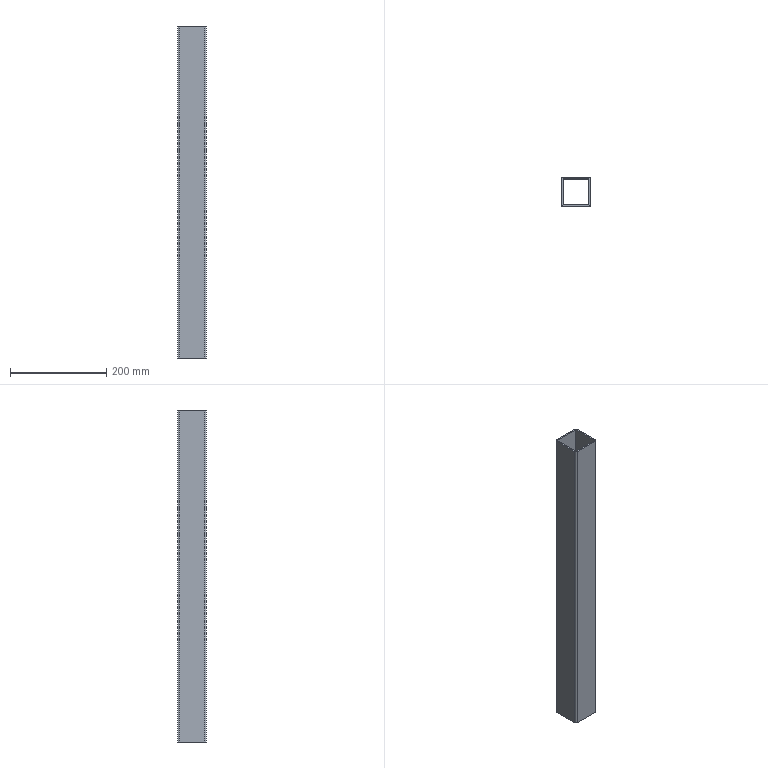Part | STEP file | X77-03104 | 1 solid | 14 faces | box 60 x 60 x 690 mm | volume 466629 mm3 | plane 10 | cylinder 4 | commonest cylinder face diameters 6 x4
STEP:
#1=CARTESIAN_POINT('',(0.,3.,690.));
#2=VERTEX_POINT('',#1);
#3=CARTESIAN_POINT('',(3.,0.,690.));
#4=VERTEX_POINT('',#3);
#5=CARTESIAN_POINT('',(3.,3.,690.));
#6=DIRECTION('',(0.,0.,1.));
#7=DIRECTION('',(1.,0.,0.));
#8=AXIS2_PLACEMENT_3D('',#5,#6,#7);
#9=CIRCLE('',#8,3.);
#10=EDGE_CURVE('',#2,#4,#9,.T.);
#11=ORIENTED_EDGE('',*,*,#10,.T.);
#12=CARTESIAN_POINT('',(57.,0.,690.));
#13=VERTEX_POINT('',#12);
#14=CARTESIAN_POINT('',(3.,0.,690.));
#15=DIRECTION('',(1.,0.,0.));
#16=VECTOR('',#15,1000.);
#17=LINE('',#14,#16);
#18=EDGE_CURVE('',#4,#13,#17,.T.);
#19=ORIENTED_EDGE('',*,*,#18,.T.);
#20=CARTESIAN_POINT('',(60.,3.,690.));
#21=VERTEX_POINT('',#20);
#22=CARTESIAN_POINT('',(57.,3.,690.));
#23=DIRECTION('',(0.,0.,1.));
#24=DIRECTION('',(1.,0.,0.));
#25=AXIS2_PLACEMENT_3D('',#22,#23,#24);
#26=CIRCLE('',#25,3.);
#27=EDGE_CURVE('',#13,#21,#26,.T.);
#28=ORIENTED_EDGE('',*,*,#27,.T.);
#29=CARTESIAN_POINT('',(60.,57.,690.));
#30=VERTEX_POINT('',#29);
#31=CARTESIAN_POINT('',(60.,3.,690.));
#32=DIRECTION('',(0.,1.,0.));
#33=VECTOR('',#32,1000.);
#34=LINE('',#31,#33);
#35=EDGE_CURVE('',#21,#30,#34,.T.);
#36=ORIENTED_EDGE('',*,*,#35,.T.);
#37=CARTESIAN_POINT('',(57.,60.,690.));
#38=VERTEX_POINT('',#37);
#39=CARTESIAN_POINT('',(57.,57.,690.));
#40=DIRECTION('',(0.,0.,1.));
#41=DIRECTION('',(1.,0.,0.));
#42=AXIS2_PLACEMENT_3D('',#39,#40,#41);
#43=CIRCLE('',#42,3.);
#44=EDGE_CURVE('',#30,#38,#43,.T.);
#45=ORIENTED_EDGE('',*,*,#44,.T.);
#46=CARTESIAN_POINT('',(3.,60.,690.));
#47=VERTEX_POINT('',#46);
#48=CARTESIAN_POINT('',(3.,60.,690.));
#49=DIRECTION('',(-1.,0.,0.));
#50=VECTOR('',#49,1000.);
#51=LINE('',#48,#50);
#52=EDGE_CURVE('',#38,#47,#51,.T.);
#53=ORIENTED_EDGE('',*,*,#52,.T.);
#54=CARTESIAN_POINT('',(0.,57.,690.));
#55=VERTEX_POINT('',#54);
#56=CARTESIAN_POINT('',(3.,57.,690.));
#57=DIRECTION('',(0.,0.,1.));
#58=DIRECTION('',(1.,0.,0.));
#59=AXIS2_PLACEMENT_3D('',#56,#57,#58);
#60=CIRCLE('',#59,3.);
#61=EDGE_CURVE('',#47,#55,#60,.T.);
#62=ORIENTED_EDGE('',*,*,#61,.T.);
#63=CARTESIAN_POINT('',(0.,3.,690.));
#64=DIRECTION('',(0.,-1.,0.));
#65=VECTOR('',#64,1000.);
#66=LINE('',#63,#65);
#67=EDGE_CURVE('',#55,#2,#66,.T.);
#68=ORIENTED_EDGE('',*,*,#67,.T.);
#69=EDGE_LOOP('',(#11,#19,#28,#36,#45,#53,#62,#68));
#70=FACE_OUTER_BOUND('',#69,.T.);
#71=CARTESIAN_POINT('',(3.,3.,690.));
#72=VERTEX_POINT('',#71);
#73=CARTESIAN_POINT('',(57.,3.,690.));
#74=VERTEX_POINT('',#73);
#75=CARTESIAN_POINT('',(3.,3.,690.));
#76=DIRECTION('',(1.,0.,0.));
#77=VECTOR('',#76,1000.);
#78=LINE('',#75,#77);
#79=EDGE_CURVE('',#72,#74,#78,.T.);
#80=ORIENTED_EDGE('',*,*,#79,.F.);
#81=CARTESIAN_POINT('',(3.,57.,690.));
#82=VERTEX_POINT('',#81);
#83=CARTESIAN_POINT('',(3.,3.,690.));
#84=DIRECTION('',(0.,-1.,0.));
#85=VECTOR('',#84,1000.);
#86=LINE('',#83,#85);
#87=EDGE_CURVE('',#82,#72,#86,.T.);
#88=ORIENTED_EDGE('',*,*,#87,.F.);
#89=CARTESIAN_POINT('',(57.,57.,690.));
#90=VERTEX_POINT('',#89);
#91=CARTESIAN_POINT('',(3.,57.,690.));
#92=DIRECTION('',(-1.,0.,0.));
#93=VECTOR('',#92,1000.);
#94=LINE('',#91,#93);
#95=EDGE_CURVE('',#90,#82,#94,.T.);
#96=ORIENTED_EDGE('',*,*,#95,.F.);
#97=CARTESIAN_POINT('',(57.,3.,690.));
#98=DIRECTION('',(0.,1.,0.));
#99=VECTOR('',#98,1000.);
#100=LINE('',#97,#99);
#101=EDGE_CURVE('',#74,#90,#100,.T.);
#102=ORIENTED_EDGE('',*,*,#101,.F.);
#103=EDGE_LOOP('',(#80,#88,#96,#102));
#104=FACE_BOUND('',#103,.T.);
#105=CARTESIAN_POINT('',(3.,3.,690.));
#106=DIRECTION('',(0.,0.,1.));
#107=DIRECTION('',(1.,0.,0.));
#108=AXIS2_PLACEMENT_3D('',#105,#106,#107);
#109=PLANE('',#108);
#110=ADVANCED_FACE('',(#70,#104),#109,.T.);
#111=CARTESIAN_POINT('',(0.,3.,0.));
#112=VERTEX_POINT('',#111);
#113=CARTESIAN_POINT('',(3.,0.,0.));
#114=VERTEX_POINT('',#113);
#115=CARTESIAN_POINT('',(3.,3.,0.));
#116=DIRECTION('',(0.,0.,1.));
#117=DIRECTION('',(1.,0.,0.));
#118=AXIS2_PLACEMENT_3D('',#115,#116,#117);
#119=CIRCLE('',#118,3.);
#120=EDGE_CURVE('',#112,#114,#119,.T.);
#121=ORIENTED_EDGE('',*,*,#120,.F.);
#122=CARTESIAN_POINT('',(0.,57.,0.));
#123=VERTEX_POINT('',#122);
#124=CARTESIAN_POINT('',(0.,3.,0.));
#125=DIRECTION('',(0.,-1.,0.));
#126=VECTOR('',#125,1000.);
#127=LINE('',#124,#126);
#128=EDGE_CURVE('',#123,#112,#127,.T.);
#129=ORIENTED_EDGE('',*,*,#128,.F.);
#130=CARTESIAN_POINT('',(3.,60.,0.));
#131=VERTEX_POINT('',#130);
#132=CARTESIAN_POINT('',(3.,57.,0.));
#133=DIRECTION('',(0.,0.,1.));
#134=DIRECTION('',(1.,0.,0.));
#135=AXIS2_PLACEMENT_3D('',#132,#133,#134);
#136=CIRCLE('',#135,3.);
#137=EDGE_CURVE('',#131,#123,#136,.T.);
#138=ORIENTED_EDGE('',*,*,#137,.F.);
#139=CARTESIAN_POINT('',(57.,60.,0.));
#140=VERTEX_POINT('',#139);
#141=CARTESIAN_POINT('',(3.,60.,0.));
#142=DIRECTION('',(-1.,0.,0.));
#143=VECTOR('',#142,1000.);
#144=LINE('',#141,#143);
#145=EDGE_CURVE('',#140,#131,#144,.T.);
#146=ORIENTED_EDGE('',*,*,#145,.F.);
#147=CARTESIAN_POINT('',(60.,57.,0.));
#148=VERTEX_POINT('',#147);
#149=CARTESIAN_POINT('',(57.,57.,0.));
#150=DIRECTION('',(0.,0.,1.));
#151=DIRECTION('',(1.,0.,0.));
#152=AXIS2_PLACEMENT_3D('',#149,#150,#151);
#153=CIRCLE('',#152,3.);
#154=EDGE_CURVE('',#148,#140,#153,.T.);
#155=ORIENTED_EDGE('',*,*,#154,.F.);
#156=CARTESIAN_POINT('',(60.,3.,0.));
#157=VERTEX_POINT('',#156);
#158=CARTESIAN_POINT('',(60.,3.,0.));
#159=DIRECTION('',(0.,1.,0.));
#160=VECTOR('',#159,1000.);
#161=LINE('',#158,#160);
#162=EDGE_CURVE('',#157,#148,#161,.T.);
#163=ORIENTED_EDGE('',*,*,#162,.F.);
#164=CARTESIAN_POINT('',(57.,0.,0.));
#165=VERTEX_POINT('',#164);
#166=CARTESIAN_POINT('',(57.,3.,0.));
#167=DIRECTION('',(0.,0.,1.));
#168=DIRECTION('',(1.,0.,0.));
#169=AXIS2_PLACEMENT_3D('',#166,#167,#168);
#170=CIRCLE('',#169,3.);
#171=EDGE_CURVE('',#165,#157,#170,.T.);
#172=ORIENTED_EDGE('',*,*,#171,.F.);
#173=CARTESIAN_POINT('',(3.,0.,0.));
#174=DIRECTION('',(1.,0.,0.));
#175=VECTOR('',#174,1000.);
#176=LINE('',#173,#175);
#177=EDGE_CURVE('',#114,#165,#176,.T.);
#178=ORIENTED_EDGE('',*,*,#177,.F.);
#179=EDGE_LOOP('',(#121,#129,#138,#146,#155,#163,#172,#178));
#180=FACE_OUTER_BOUND('',#179,.T.);
#181=CARTESIAN_POINT('',(3.,57.,0.));
#182=VERTEX_POINT('',#181);
#183=CARTESIAN_POINT('',(3.,3.,0.));
#184=VERTEX_POINT('',#183);
#185=CARTESIAN_POINT('',(3.,3.,0.));
#186=DIRECTION('',(0.,-1.,0.));
#187=VECTOR('',#186,1000.);
#188=LINE('',#185,#187);
#189=EDGE_CURVE('',#182,#184,#188,.T.);
#190=ORIENTED_EDGE('',*,*,#189,.T.);
#191=CARTESIAN_POINT('',(57.,3.,0.));
#192=VERTEX_POINT('',#191);
#193=CARTESIAN_POINT('',(3.,3.,0.));
#194=DIRECTION('',(1.,0.,0.));
#195=VECTOR('',#194,1000.);
#196=LINE('',#193,#195);
#197=EDGE_CURVE('',#184,#192,#196,.T.);
#198=ORIENTED_EDGE('',*,*,#197,.T.);
#199=CARTESIAN_POINT('',(57.,57.,0.));
#200=VERTEX_POINT('',#199);
#201=CARTESIAN_POINT('',(57.,3.,0.));
#202=DIRECTION('',(0.,1.,0.));
#203=VECTOR('',#202,1000.);
#204=LINE('',#201,#203);
#205=EDGE_CURVE('',#192,#200,#204,.T.);
#206=ORIENTED_EDGE('',*,*,#205,.T.);
#207=CARTESIAN_POINT('',(3.,57.,0.));
#208=DIRECTION('',(-1.,0.,0.));
#209=VECTOR('',#208,1000.);
#210=LINE('',#207,#209);
#211=EDGE_CURVE('',#200,#182,#210,.T.);
#212=ORIENTED_EDGE('',*,*,#211,.T.);
#213=EDGE_LOOP('',(#190,#198,#206,#212));
#214=FACE_BOUND('',#213,.T.);
#215=CARTESIAN_POINT('',(3.,3.,0.));
#216=DIRECTION('',(0.,0.,1.));
#217=DIRECTION('',(1.,0.,0.));
#218=AXIS2_PLACEMENT_3D('',#215,#216,#217);
#219=PLANE('',#218);
#220=ADVANCED_FACE('',(#180,#214),#219,.F.);
#221=ORIENTED_EDGE('',*,*,#120,.T.);
#222=CARTESIAN_POINT('',(3.,0.,690.));
#223=DIRECTION('',(0.,0.,-1.));
#224=VECTOR('',#223,1000.);
#225=LINE('',#222,#224);
#226=EDGE_CURVE('',#4,#114,#225,.T.);
#227=ORIENTED_EDGE('',*,*,#226,.F.);
#228=ORIENTED_EDGE('',*,*,#10,.F.);
#229=CARTESIAN_POINT('',(0.,3.,690.));
#230=DIRECTION('',(0.,0.,-1.));
#231=VECTOR('',#230,1000.);
#232=LINE('',#229,#231);
#233=EDGE_CURVE('',#2,#112,#232,.T.);
#234=ORIENTED_EDGE('',*,*,#233,.T.);
#235=EDGE_LOOP('',(#221,#227,#228,#234));
#236=FACE_OUTER_BOUND('',#235,.T.);
#237=CARTESIAN_POINT('',(3.,3.,690.));
#238=DIRECTION('',(0.,0.,-1.));
#239=DIRECTION('',(-1.,0.,0.));
#240=AXIS2_PLACEMENT_3D('',#237,#238,#239);
#241=CYLINDRICAL_SURFACE('',#240,3.);
#242=ADVANCED_FACE('',(#236),#241,.T.);
#243=ORIENTED_EDGE('',*,*,#177,.T.);
#244=CARTESIAN_POINT('',(57.,0.,690.));
#245=DIRECTION('',(0.,0.,-1.));
#246=VECTOR('',#245,1000.);
#247=LINE('',#244,#246);
#248=EDGE_CURVE('',#13,#165,#247,.T.);
#249=ORIENTED_EDGE('',*,*,#248,.F.);
#250=ORIENTED_EDGE('',*,*,#18,.F.);
#251=ORIENTED_EDGE('',*,*,#226,.T.);
#252=EDGE_LOOP('',(#243,#249,#250,#251));
#253=FACE_OUTER_BOUND('',#252,.T.);
#254=CARTESIAN_POINT('',(3.,0.,690.));
#255=DIRECTION('',(0.,1.,0.));
#256=DIRECTION('',(0.,0.,1.));
#257=AXIS2_PLACEMENT_3D('',#254,#255,#256);
#258=PLANE('',#257);
#259=ADVANCED_FACE('',(#253),#258,.F.);
#260=ORIENTED_EDGE('',*,*,#171,.T.);
#261=CARTESIAN_POINT('',(60.,3.,690.));
#262=DIRECTION('',(0.,0.,-1.));
#263=VECTOR('',#262,1000.);
#264=LINE('',#261,#263);
#265=EDGE_CURVE('',#21,#157,#264,.T.);
#266=ORIENTED_EDGE('',*,*,#265,.F.);
#267=ORIENTED_EDGE('',*,*,#27,.F.);
#268=ORIENTED_EDGE('',*,*,#248,.T.);
#269=EDGE_LOOP('',(#260,#266,#267,#268));
#270=FACE_OUTER_BOUND('',#269,.T.);
#271=CARTESIAN_POINT('',(57.,3.,690.));
#272=DIRECTION('',(0.,0.,-1.));
#273=DIRECTION('',(-1.,0.,0.));
#274=AXIS2_PLACEMENT_3D('',#271,#272,#273);
#275=CYLINDRICAL_SURFACE('',#274,3.);
#276=ADVANCED_FACE('',(#270),#275,.T.);
#277=ORIENTED_EDGE('',*,*,#162,.T.);
#278=CARTESIAN_POINT('',(60.,57.,690.));
#279=DIRECTION('',(0.,0.,-1.));
#280=VECTOR('',#279,1000.);
#281=LINE('',#278,#280);
#282=EDGE_CURVE('',#30,#148,#281,.T.);
#283=ORIENTED_EDGE('',*,*,#282,.F.);
#284=ORIENTED_EDGE('',*,*,#35,.F.);
#285=ORIENTED_EDGE('',*,*,#265,.T.);
#286=EDGE_LOOP('',(#277,#283,#284,#285));
#287=FACE_OUTER_BOUND('',#286,.T.);
#288=CARTESIAN_POINT('',(60.,3.,690.));
#289=DIRECTION('',(-1.,0.,0.));
#290=DIRECTION('',(0.,0.,1.));
#291=AXIS2_PLACEMENT_3D('',#288,#289,#290);
#292=PLANE('',#291);
#293=ADVANCED_FACE('',(#287),#292,.F.);
#294=ORIENTED_EDGE('',*,*,#154,.T.);
#295=CARTESIAN_POINT('',(57.,60.,690.));
#296=DIRECTION('',(0.,0.,-1.));
#297=VECTOR('',#296,1000.);
#298=LINE('',#295,#297);
#299=EDGE_CURVE('',#38,#140,#298,.T.);
#300=ORIENTED_EDGE('',*,*,#299,.F.);
#301=ORIENTED_EDGE('',*,*,#44,.F.);
#302=ORIENTED_EDGE('',*,*,#282,.T.);
#303=EDGE_LOOP('',(#294,#300,#301,#302));
#304=FACE_OUTER_BOUND('',#303,.T.);
#305=CARTESIAN_POINT('',(57.,57.,690.));
#306=DIRECTION('',(0.,0.,-1.));
#307=DIRECTION('',(-1.,0.,0.));
#308=AXIS2_PLACEMENT_3D('',#305,#306,#307);
#309=CYLINDRICAL_SURFACE('',#308,3.);
#310=ADVANCED_FACE('',(#304),#309,.T.);
#311=ORIENTED_EDGE('',*,*,#145,.T.);
#312=CARTESIAN_POINT('',(3.,60.,690.));
#313=DIRECTION('',(0.,0.,-1.));
#314=VECTOR('',#313,1000.);
#315=LINE('',#312,#314);
#316=EDGE_CURVE('',#47,#131,#315,.T.);
#317=ORIENTED_EDGE('',*,*,#316,.F.);
#318=ORIENTED_EDGE('',*,*,#52,.F.);
#319=ORIENTED_EDGE('',*,*,#299,.T.);
#320=EDGE_LOOP('',(#311,#317,#318,#319));
#321=FACE_OUTER_BOUND('',#320,.T.);
#322=CARTESIAN_POINT('',(3.,60.,690.));
#323=DIRECTION('',(0.,-1.,0.));
#324=DIRECTION('',(0.,0.,-1.));
#325=AXIS2_PLACEMENT_3D('',#322,#323,#324);
#326=PLANE('',#325);
#327=ADVANCED_FACE('',(#321),#326,.F.);
#328=ORIENTED_EDGE('',*,*,#137,.T.);
#329=CARTESIAN_POINT('',(0.,57.,690.));
#330=DIRECTION('',(0.,0.,-1.));
#331=VECTOR('',#330,1000.);
#332=LINE('',#329,#331);
#333=EDGE_CURVE('',#55,#123,#332,.T.);
#334=ORIENTED_EDGE('',*,*,#333,.F.);
#335=ORIENTED_EDGE('',*,*,#61,.F.);
#336=ORIENTED_EDGE('',*,*,#316,.T.);
#337=EDGE_LOOP('',(#328,#334,#335,#336));
#338=FACE_OUTER_BOUND('',#337,.T.);
#339=CARTESIAN_POINT('',(3.,57.,690.));
#340=DIRECTION('',(0.,0.,-1.));
#341=DIRECTION('',(-1.,0.,0.));
#342=AXIS2_PLACEMENT_3D('',#339,#340,#341);
#343=CYLINDRICAL_SURFACE('',#342,3.);
#344=ADVANCED_FACE('',(#338),#343,.T.);
#345=ORIENTED_EDGE('',*,*,#128,.T.);
#346=ORIENTED_EDGE('',*,*,#233,.F.);
#347=ORIENTED_EDGE('',*,*,#67,.F.);
#348=ORIENTED_EDGE('',*,*,#333,.T.);
#349=EDGE_LOOP('',(#345,#346,#347,#348));
#350=FACE_OUTER_BOUND('',#349,.T.);
#351=CARTESIAN_POINT('',(0.,3.,690.));
#352=DIRECTION('',(1.,0.,0.));
#353=DIRECTION('',(0.,0.,-1.));
#354=AXIS2_PLACEMENT_3D('',#351,#352,#353);
#355=PLANE('',#354);
#356=ADVANCED_FACE('',(#350),#355,.F.);
#357=ORIENTED_EDGE('',*,*,#189,.F.);
#358=CARTESIAN_POINT('',(3.,57.,690.));
#359=DIRECTION('',(0.,0.,-1.));
#360=VECTOR('',#359,1000.);
#361=LINE('',#358,#360);
#362=EDGE_CURVE('',#82,#182,#361,.T.);
#363=ORIENTED_EDGE('',*,*,#362,.F.);
#364=ORIENTED_EDGE('',*,*,#87,.T.);
#365=CARTESIAN_POINT('',(3.,3.,690.));
#366=DIRECTION('',(0.,0.,-1.));
#367=VECTOR('',#366,1000.);
#368=LINE('',#365,#367);
#369=EDGE_CURVE('',#72,#184,#368,.T.);
#370=ORIENTED_EDGE('',*,*,#369,.T.);
#371=EDGE_LOOP('',(#357,#363,#364,#370));
#372=FACE_OUTER_BOUND('',#371,.T.);
#373=CARTESIAN_POINT('',(3.,3.,690.));
#374=DIRECTION('',(1.,0.,0.));
#375=DIRECTION('',(0.,0.,-1.));
#376=AXIS2_PLACEMENT_3D('',#373,#374,#375);
#377=PLANE('',#376);
#378=ADVANCED_FACE('',(#372),#377,.T.);
#379=ORIENTED_EDGE('',*,*,#197,.F.);
#380=ORIENTED_EDGE('',*,*,#369,.F.);
#381=ORIENTED_EDGE('',*,*,#79,.T.);
#382=CARTESIAN_POINT('',(57.,3.,690.));
#383=DIRECTION('',(0.,0.,-1.));
#384=VECTOR('',#383,1000.);
#385=LINE('',#382,#384);
#386=EDGE_CURVE('',#74,#192,#385,.T.);
#387=ORIENTED_EDGE('',*,*,#386,.T.);
#388=EDGE_LOOP('',(#379,#380,#381,#387));
#389=FACE_OUTER_BOUND('',#388,.T.);
#390=CARTESIAN_POINT('',(3.,3.,690.));
#391=DIRECTION('',(0.,1.,0.));
#392=DIRECTION('',(0.,0.,1.));
#393=AXIS2_PLACEMENT_3D('',#390,#391,#392);
#394=PLANE('',#393);
#395=ADVANCED_FACE('',(#389),#394,.T.);
#396=ORIENTED_EDGE('',*,*,#205,.F.);
#397=ORIENTED_EDGE('',*,*,#386,.F.);
#398=ORIENTED_EDGE('',*,*,#101,.T.);
#399=CARTESIAN_POINT('',(57.,57.,690.));
#400=DIRECTION('',(0.,0.,-1.));
#401=VECTOR('',#400,1000.);
#402=LINE('',#399,#401);
#403=EDGE_CURVE('',#90,#200,#402,.T.);
#404=ORIENTED_EDGE('',*,*,#403,.T.);
#405=EDGE_LOOP('',(#396,#397,#398,#404));
#406=FACE_OUTER_BOUND('',#405,.T.);
#407=CARTESIAN_POINT('',(57.,3.,690.));
#408=DIRECTION('',(-1.,0.,0.));
#409=DIRECTION('',(0.,0.,1.));
#410=AXIS2_PLACEMENT_3D('',#407,#408,#409);
#411=PLANE('',#410);
#412=ADVANCED_FACE('',(#406),#411,.T.);
#413=ORIENTED_EDGE('',*,*,#211,.F.);
#414=ORIENTED_EDGE('',*,*,#403,.F.);
#415=ORIENTED_EDGE('',*,*,#95,.T.);
#416=ORIENTED_EDGE('',*,*,#362,.T.);
#417=EDGE_LOOP('',(#413,#414,#415,#416));
#418=FACE_OUTER_BOUND('',#417,.T.);
#419=CARTESIAN_POINT('',(3.,57.,690.));
#420=DIRECTION('',(0.,-1.,0.));
#421=DIRECTION('',(0.,0.,-1.));
#422=AXIS2_PLACEMENT_3D('',#419,#420,#421);
#423=PLANE('',#422);
#424=ADVANCED_FACE('',(#418),#423,.T.);
#425=CLOSED_SHELL('',(#110,#220,#242,#259,#276,#293,#310,#327,#344,#356,#378,#395,#412,#424));
#426=MANIFOLD_SOLID_BREP('',#425);
#427=CARTESIAN_POINT('',(0.,0.,0.));
#428=DIRECTION('',(0.,0.,1.));
#429=DIRECTION('',(1.,0.,0.));
#430=AXIS2_PLACEMENT_3D('',#427,#428,#429);
#431=(LENGTH_UNIT()NAMED_UNIT(*)SI_UNIT(.MILLI.,.METRE.));
#432=UNCERTAINTY_MEASURE_WITH_UNIT(LENGTH_MEASURE(0.00001),#431,'','');
#433=(NAMED_UNIT(*)PLANE_ANGLE_UNIT()SI_UNIT($,.RADIAN.));
#434=(NAMED_UNIT(*)SI_UNIT($,.STERADIAN.)SOLID_ANGLE_UNIT());
#435=(GEOMETRIC_REPRESENTATION_CONTEXT(3)GLOBAL_UNCERTAINTY_ASSIGNED_CONTEXT((#432))GLOBAL_UNIT_ASSIGNED_CONTEXT((#431,#433,#434))REPRESENTATION_CONTEXT('',''));
#436=ADVANCED_BREP_SHAPE_REPRESENTATION('',(#426,#430),#435);